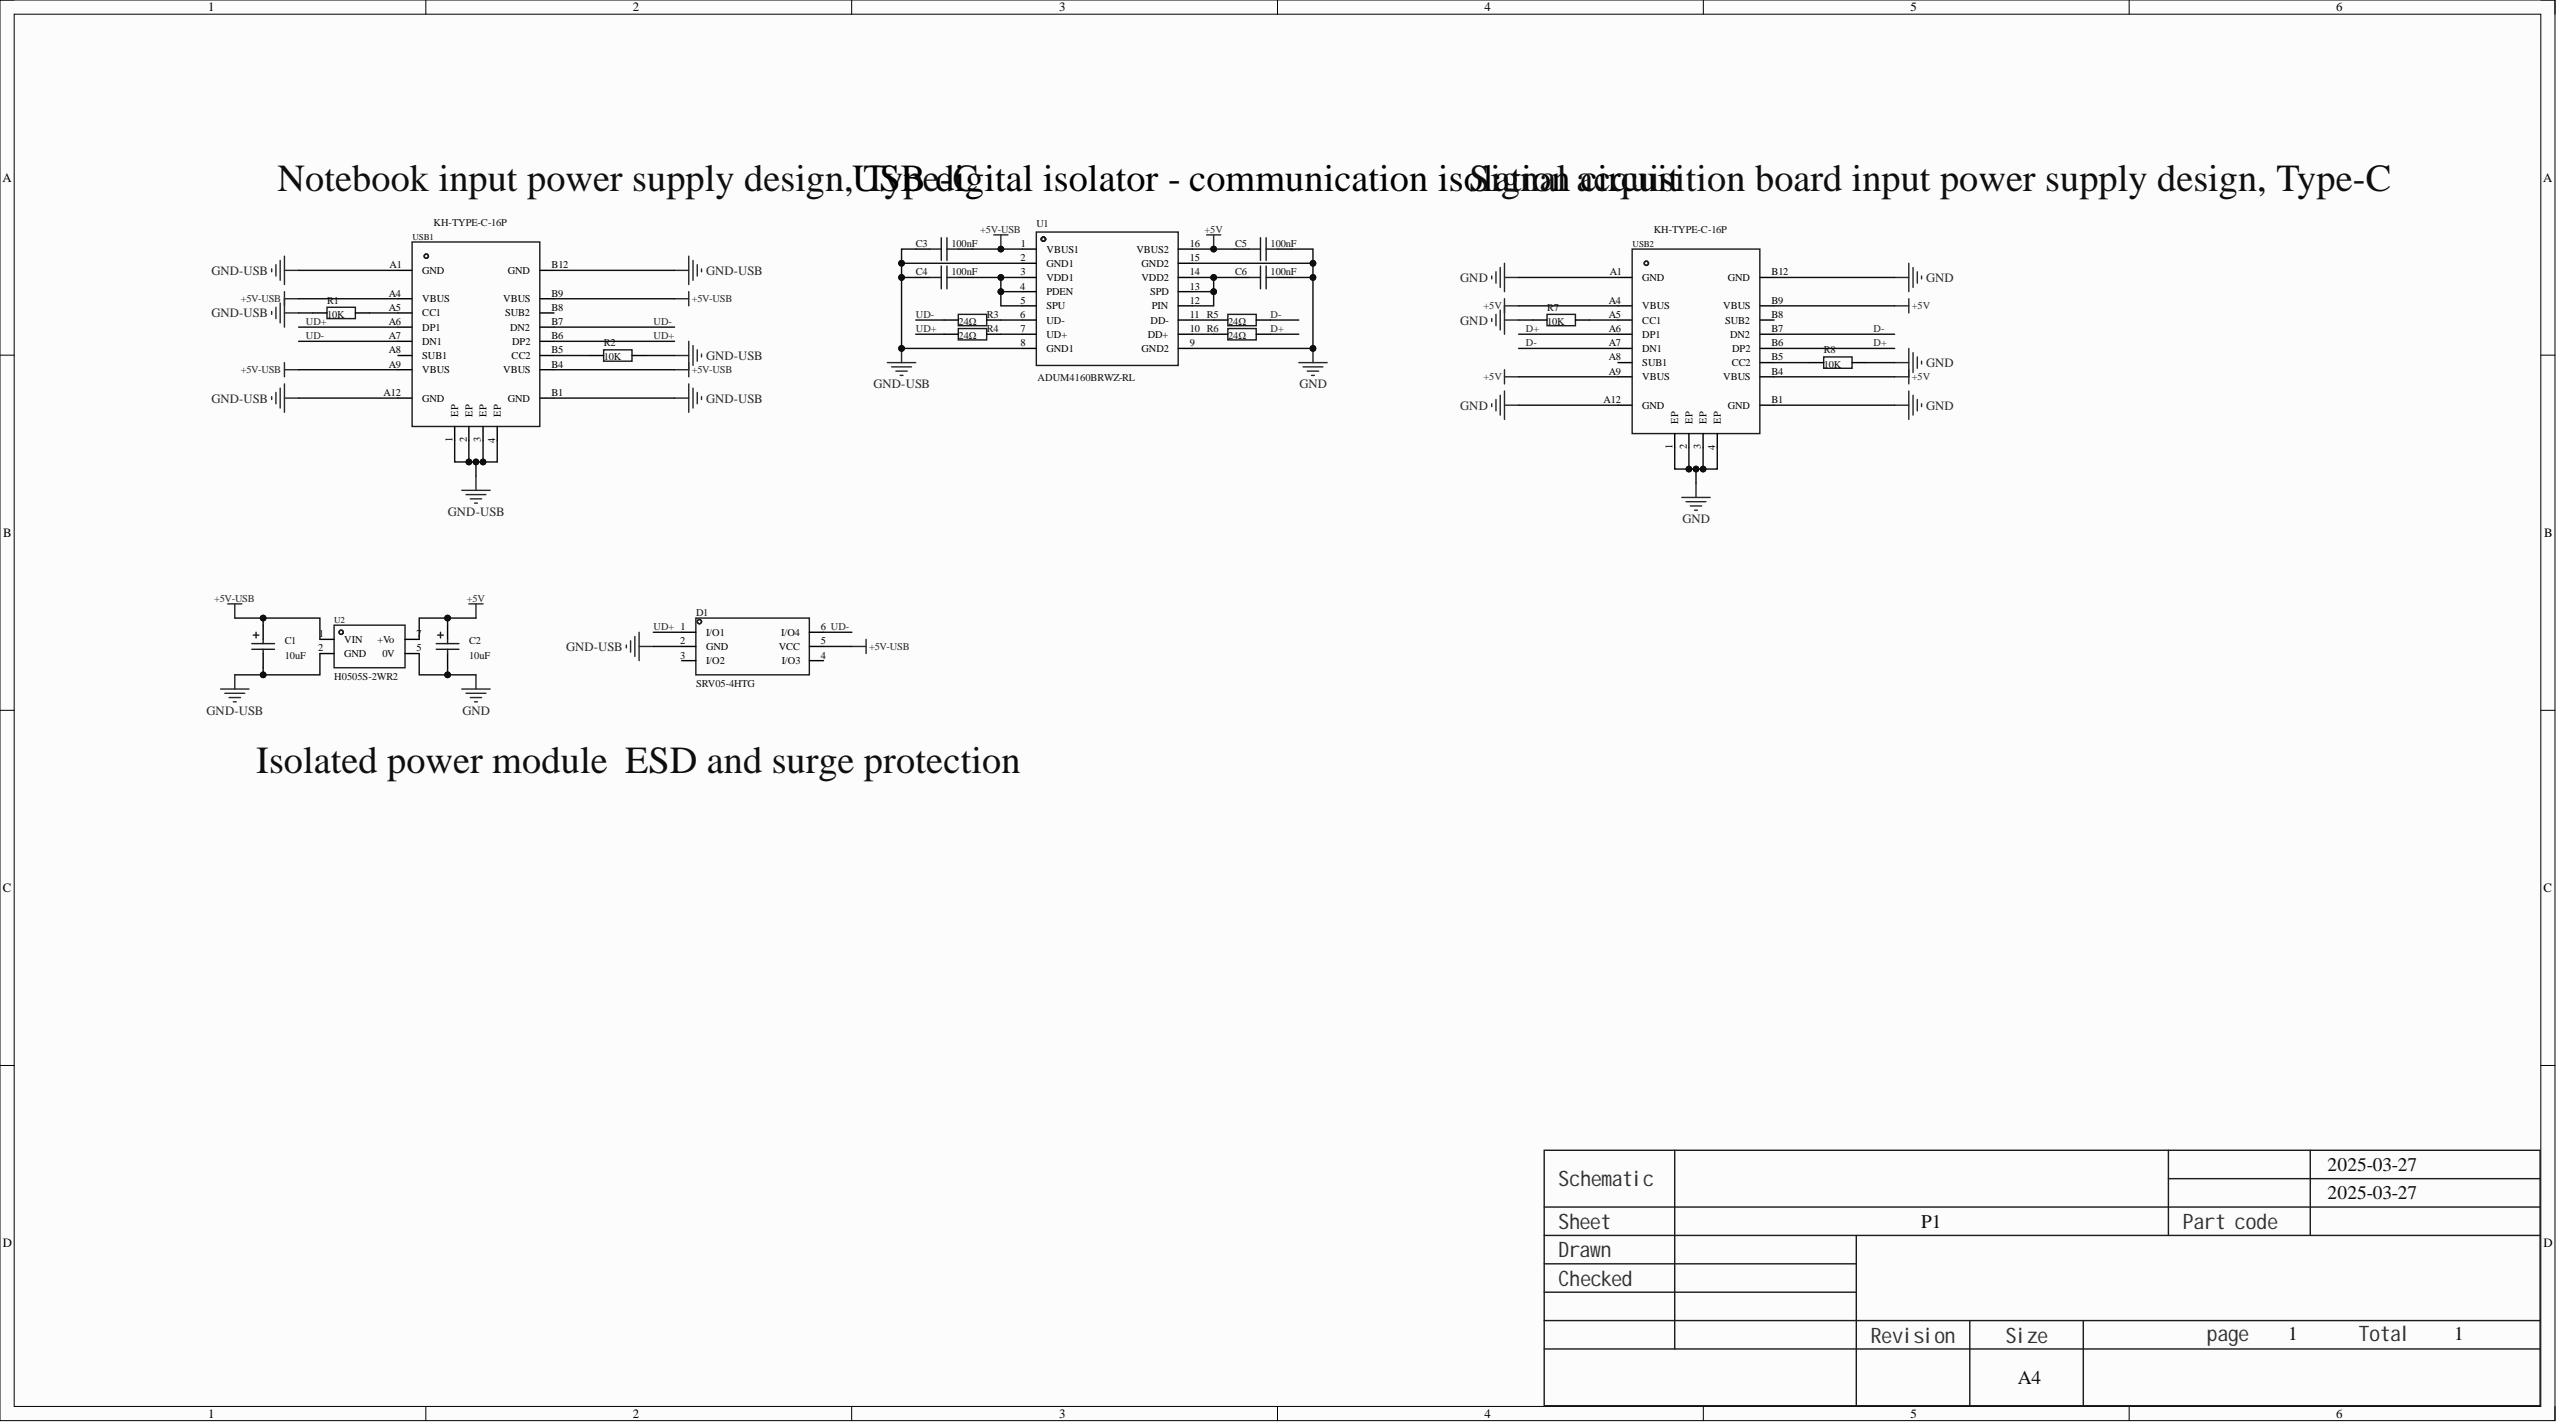Circuit board | Altium Designer | 19 parts | 18 nets
Bill of materials:
Comment,Description,Designator,Footprint,LibRef,Quantity
"10uF","Capacitance: 10uF; Tolerance: ±10%; Rated voltage: 16V; ESR: 3Ω@100kHz;","C1, C2","CAP-SMD_L3.2-W1.6-RD-C7171","TAJA106K016RNJ","2"
"100nF","Capacitance: 100nF; Tolerance: ±10%; Rated voltage: 50V; Dielectric (temperature coefficient): X7R;","C3, C4, C5, C6","C0603","CC0603KRX7R9BB104","4"
"SRV05-4HTG","Reverse stand-off voltage (Vrwm): 6V@Max; Breakdown voltage: -; Peak pulse current (Ipp)@10/1000µs: -; Max clamping voltage: 15V; Peak pulse power (Ppp)@10/1000µs: 150W;","D1","SOT-23-6_L2.9-W1.6-P0.95-LS2.8-BL","SRV05-4HTG_C151305","1"
"10K","","R1, R2, R7, R8","R0603","Res_0805","4"
"24Ω","","R3, R4, R5, R6","R0603","RC0603FR-0724RL","4"
"ADUM4160BRWZ-RL","Isolator technology: Magnetic Coupling; Type: USB; Channels: 1; Channel type: Bidirectional; Isolation voltage: 5000Vrms; Data rate: 12Mbps;","U1","SOIC-16_L10.3-W7.5-P1.27-LS10.3-BL","ADUM4160BRWZ-RL_C57791","1"
"H0505S-2WR2","Converter type: DC-DC; Input voltage (DC): 4.5V~5.5V; Output voltage: 5V; Output current (max): 400mA; Output power: 2W; Efficiency: 88%;","U2","PWRM-TH_EVISUN_HXXXXS-2WR2","H0505S-2WR2","1"
"KH-TYPE-C-16P","Type-C receptacle 16PIN, vertical, four-corner SMT, no hold-down tabs","USB1, USB2","USB-C-SMD_KH-TYPE-C-16P","KH-TYPE-C-16P","2"
Netlist (Protel format):
[
C1
CAP-SMD_L3.2-W1.6-RD-C7171
10uF



]
[
C2
CAP-SMD_L3.2-W1.6-RD-C7171
10uF



]
[
C3
C0603
100nF



]
[
C4
C0603
100nF



]
[
C5
C0603
100nF



]
[
C6
C0603
100nF



]
[
D1
SOT-23-6_L2.9-W1.6-P0.95-LS2.8-BL
SRV05-4HTG



]
[
R1
R0603
10K



]
[
R2
R0603
10K



]
[
R3
R0603
24Ω



]
[
R4
R0603
24Ω



]
[
R5
R0603
24Ω



]
[
R6
R0603
24Ω



]
[
R7
R0603
10K



]
[
R8
R0603
10K



]
[
U1
SOIC-16_L10.3-W7.5-P1.27-LS10.3-BL
ADUM4160BRWZ-RL



]
[
U2
PWRM-TH_EVISUN_HXXXXS-2WR2
H0505S-2WR2



]
[
USB1
USB-C-SMD_KH-TYPE-C-16P
KH-TYPE-C-16P



]
[
USB2
USB-C-SMD_KH-TYPE-C-16P
KH-TYPE-C-16P



]
(
UD-
D1-6
R3-1
USB1-A7
USB1-B7
)
(
UD+
D1-1
R4-1
USB1-A6
USB1-B6
)
(
NetR8_2
R8-2
USB2-B5
)
(
NetR7_1
R7-1
USB2-A5
)
(
NetR6_1
R6-1
U1-10
)
(
NetR5_1
R5-1
U1-11
)
(
NetR4_2
R4-2
U1-7
)
(
NetR3_2
R3-2
U1-6
)
(
NetR2_2
R2-2
USB1-B5
)
(
NetR1_1
R1-1
USB1-A5
)
(
NetC6_1
C6-1
U1-12
U1-13
U1-14
)
(
NetC4_2
C4-2
U1-3
U1-4
U1-5
)
(
GND-USB
C1-2
C3-1
C4-1
D1-2
R1-2
R2-1
U1-2
U1-8
U2-2
USB1-1
USB1-2
USB1-3
USB1-4
USB1-A1
USB1-A12
USB1-B1
USB1-B12
)
(
GND
C2-2
C5-2
C6-2
R7-2
R8-1
U1-9
U1-15
U2-5
USB2-1
USB2-2
USB2-3
USB2-4
USB2-A1
USB2-A12
USB2-B1
USB2-B12
)
(
D-
R5-2
USB2-A7
USB2-B7
)
(
D+
R6-2
USB2-A6
USB2-B6
)
(
+5V-USB
C1-1
C3-2
D1-5
U1-1
U2-1
USB1-A4
USB1-A9
USB1-B4
USB1-B9
)
(
+5V
C2-1
C5-1
U1-16
U2-7
USB2-A4
USB2-A9
USB2-B4
USB2-B9
)